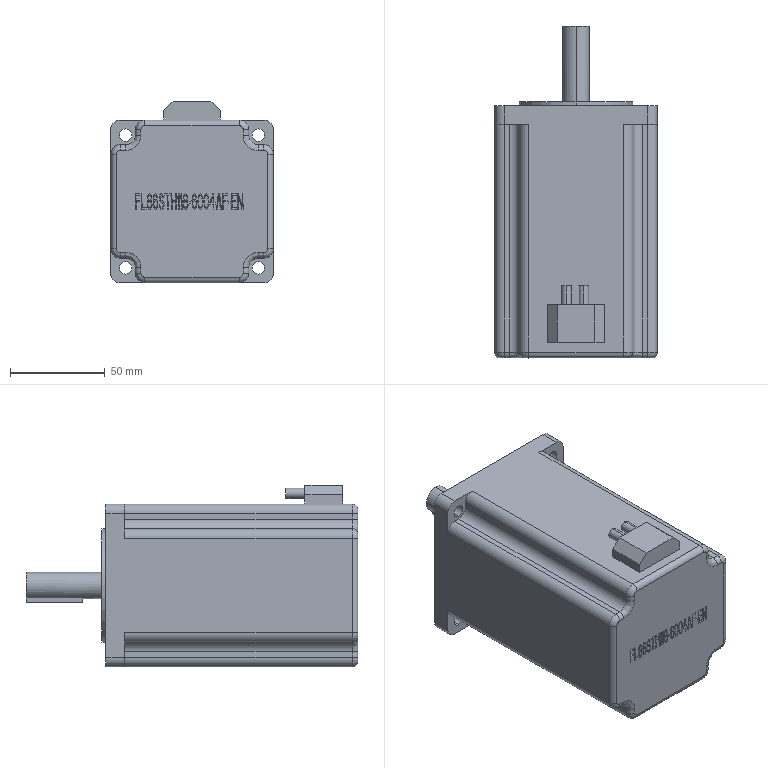Part | STEP file | 11-FL86STH118-6004AF-EN11 | 1 solid | 628 faces | box 85.85 x 175 x 95.85 mm | volume 910022 mm3 | plane 572 | cylinder 44 | torus 8 | spline 4 | commonest cylinder face diameters 10 x16 6 x12 6.5 x8 5.405 x4 14 x2 60 x2